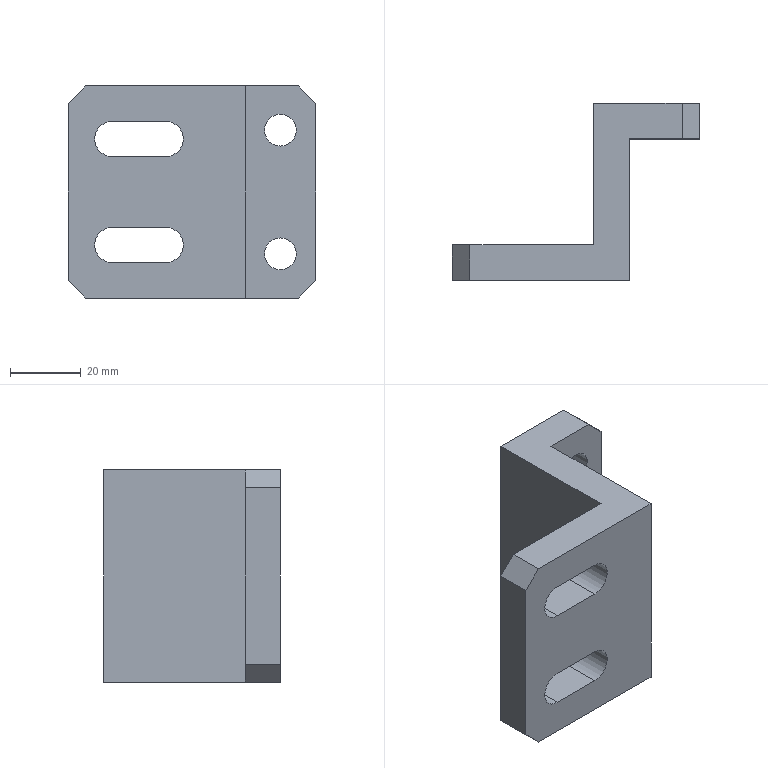Part | SolidWorks | features HoleWzd 2, Chamfer 1, Extrusion 1 | 1 solid | 26 faces | box 70 x 50 x 60 mm | volume 59657 mm3 | plane 18 | cylinder 8 | commonest cylinder face diameters 9 x4 10 x4
STEP:
#1=CARTESIAN_POINT('',(10.,40.,-22.));
#2=VERTEX_POINT('',#1);
#3=CARTESIAN_POINT('',(10.,40.,-13.));
#4=VERTEX_POINT('',#3);
#5=CARTESIAN_POINT('',(10.,40.,-17.5));
#6=DIRECTION('',(0.,1.,0.));
#7=DIRECTION('',(0.,0.,1.));
#8=AXIS2_PLACEMENT_3D('',#5,#6,#7);
#9=CIRCLE('',#8,4.5);
#10=EDGE_CURVE('',#2,#4,#9,.T.);
#11=ORIENTED_EDGE('',*,*,#10,.F.);
#12=CARTESIAN_POINT('',(10.,50.,-22.));
#13=VERTEX_POINT('',#12);
#14=CARTESIAN_POINT('',(10.,50.,-22.));
#15=DIRECTION('',(0.,1.,0.));
#16=VECTOR('',#15,1000.);
#17=LINE('',#14,#16);
#18=EDGE_CURVE('',#2,#13,#17,.T.);
#19=ORIENTED_EDGE('',*,*,#18,.T.);
#20=CARTESIAN_POINT('',(10.,50.,-13.));
#21=VERTEX_POINT('',#20);
#22=CARTESIAN_POINT('',(10.,50.,-17.5));
#23=DIRECTION('',(0.,1.,0.));
#24=DIRECTION('',(0.,0.,1.));
#25=AXIS2_PLACEMENT_3D('',#22,#23,#24);
#26=CIRCLE('',#25,4.5);
#27=EDGE_CURVE('',#13,#21,#26,.T.);
#28=ORIENTED_EDGE('',*,*,#27,.T.);
#29=CARTESIAN_POINT('',(10.,50.,-13.));
#30=DIRECTION('',(0.,1.,0.));
#31=VECTOR('',#30,1000.);
#32=LINE('',#29,#31);
#33=EDGE_CURVE('',#4,#21,#32,.T.);
#34=ORIENTED_EDGE('',*,*,#33,.F.);
#35=EDGE_LOOP('',(#11,#19,#28,#34));
#36=FACE_OUTER_BOUND('',#35,.T.);
#37=CARTESIAN_POINT('',(10.,50.,-17.5));
#38=DIRECTION('',(0.,1.,0.));
#39=DIRECTION('',(0.,0.,1.));
#40=AXIS2_PLACEMENT_3D('',#37,#38,#39);
#41=CYLINDRICAL_SURFACE('',#40,4.5);
#42=ADVANCED_FACE('',(#36),#41,.F.);
#43=CARTESIAN_POINT('',(10.,40.,13.));
#44=VERTEX_POINT('',#43);
#45=CARTESIAN_POINT('',(10.,40.,22.));
#46=VERTEX_POINT('',#45);
#47=CARTESIAN_POINT('',(10.,40.,17.5));
#48=DIRECTION('',(0.,1.,0.));
#49=DIRECTION('',(0.,0.,1.));
#50=AXIS2_PLACEMENT_3D('',#47,#48,#49);
#51=CIRCLE('',#50,4.5);
#52=EDGE_CURVE('',#44,#46,#51,.T.);
#53=ORIENTED_EDGE('',*,*,#52,.F.);
#54=CARTESIAN_POINT('',(10.,50.,13.));
#55=VERTEX_POINT('',#54);
#56=CARTESIAN_POINT('',(10.,50.,13.));
#57=DIRECTION('',(0.,1.,0.));
#58=VECTOR('',#57,1000.);
#59=LINE('',#56,#58);
#60=EDGE_CURVE('',#44,#55,#59,.T.);
#61=ORIENTED_EDGE('',*,*,#60,.T.);
#62=CARTESIAN_POINT('',(10.,50.,22.));
#63=VERTEX_POINT('',#62);
#64=CARTESIAN_POINT('',(10.,50.,17.5));
#65=DIRECTION('',(0.,1.,0.));
#66=DIRECTION('',(0.,0.,1.));
#67=AXIS2_PLACEMENT_3D('',#64,#65,#66);
#68=CIRCLE('',#67,4.5);
#69=EDGE_CURVE('',#55,#63,#68,.T.);
#70=ORIENTED_EDGE('',*,*,#69,.T.);
#71=CARTESIAN_POINT('',(10.,50.,22.));
#72=DIRECTION('',(0.,1.,0.));
#73=VECTOR('',#72,1000.);
#74=LINE('',#71,#73);
#75=EDGE_CURVE('',#46,#63,#74,.T.);
#76=ORIENTED_EDGE('',*,*,#75,.F.);
#77=EDGE_LOOP('',(#53,#61,#70,#76));
#78=FACE_OUTER_BOUND('',#77,.T.);
#79=CARTESIAN_POINT('',(10.,50.,17.5));
#80=DIRECTION('',(0.,1.,0.));
#81=DIRECTION('',(0.,0.,1.));
#82=AXIS2_PLACEMENT_3D('',#79,#80,#81);
#83=CYLINDRICAL_SURFACE('',#82,4.5);
#84=ADVANCED_FACE('',(#78),#83,.F.);
#85=CARTESIAN_POINT('',(-45.,0.,30.));
#86=VERTEX_POINT('',#85);
#87=CARTESIAN_POINT('',(0.,0.,30.));
#88=VERTEX_POINT('',#87);
#89=CARTESIAN_POINT('',(0.,0.,30.));
#90=DIRECTION('',(1.,0.,0.));
#91=VECTOR('',#90,1000.);
#92=LINE('',#89,#91);
#93=EDGE_CURVE('',#86,#88,#92,.T.);
#94=ORIENTED_EDGE('',*,*,#93,.F.);
#95=CARTESIAN_POINT('',(-50.,0.,25.));
#96=VERTEX_POINT('',#95);
#97=CARTESIAN_POINT('',(-45.,0.,30.));
#98=DIRECTION('',(-0.7071,0.,-0.7071));
#99=VECTOR('',#98,1000.);
#100=LINE('',#97,#99);
#101=EDGE_CURVE('',#86,#96,#100,.T.);
#102=ORIENTED_EDGE('',*,*,#101,.T.);
#103=CARTESIAN_POINT('',(-50.,0.,-25.));
#104=VERTEX_POINT('',#103);
#105=CARTESIAN_POINT('',(-50.,0.,30.));
#106=DIRECTION('',(0.,0.,-1.));
#107=VECTOR('',#106,1000.);
#108=LINE('',#105,#107);
#109=EDGE_CURVE('',#96,#104,#108,.T.);
#110=ORIENTED_EDGE('',*,*,#109,.T.);
#111=CARTESIAN_POINT('',(-45.,0.,-30.));
#112=VERTEX_POINT('',#111);
#113=CARTESIAN_POINT('',(-50.,0.,-25.));
#114=DIRECTION('',(0.7071,0.,-0.7071));
#115=VECTOR('',#114,1000.);
#116=LINE('',#113,#115);
#117=EDGE_CURVE('',#104,#112,#116,.T.);
#118=ORIENTED_EDGE('',*,*,#117,.T.);
#119=CARTESIAN_POINT('',(0.,0.,-30.));
#120=VERTEX_POINT('',#119);
#121=CARTESIAN_POINT('',(0.,0.,-30.));
#122=DIRECTION('',(1.,0.,0.));
#123=VECTOR('',#122,1000.);
#124=LINE('',#121,#123);
#125=EDGE_CURVE('',#112,#120,#124,.T.);
#126=ORIENTED_EDGE('',*,*,#125,.T.);
#127=CARTESIAN_POINT('',(0.,0.,30.));
#128=DIRECTION('',(0.,0.,-1.));
#129=VECTOR('',#128,1000.);
#130=LINE('',#127,#129);
#131=EDGE_CURVE('',#88,#120,#130,.T.);
#132=ORIENTED_EDGE('',*,*,#131,.F.);
#133=EDGE_LOOP('',(#94,#102,#110,#118,#126,#132));
#134=FACE_OUTER_BOUND('',#133,.T.);
#135=CARTESIAN_POINT('',(-37.5,0.,10.));
#136=VERTEX_POINT('',#135);
#137=CARTESIAN_POINT('',(-22.5,0.,10.));
#138=VERTEX_POINT('',#137);
#139=CARTESIAN_POINT('',(-37.5,0.,10.));
#140=DIRECTION('',(1.,0.,0.));
#141=VECTOR('',#140,1000.);
#142=LINE('',#139,#141);
#143=EDGE_CURVE('',#136,#138,#142,.T.);
#144=ORIENTED_EDGE('',*,*,#143,.F.);
#145=CARTESIAN_POINT('',(-37.5,0.,20.));
#146=VERTEX_POINT('',#145);
#147=CARTESIAN_POINT('',(-37.5,0.,15.));
#148=DIRECTION('',(0.,1.,0.));
#149=DIRECTION('',(0.,0.,1.));
#150=AXIS2_PLACEMENT_3D('',#147,#148,#149);
#151=CIRCLE('',#150,5.);
#152=EDGE_CURVE('',#136,#146,#151,.T.);
#153=ORIENTED_EDGE('',*,*,#152,.T.);
#154=CARTESIAN_POINT('',(-22.5,0.,20.));
#155=VERTEX_POINT('',#154);
#156=CARTESIAN_POINT('',(-37.5,0.,20.));
#157=DIRECTION('',(1.,0.,0.));
#158=VECTOR('',#157,1000.);
#159=LINE('',#156,#158);
#160=EDGE_CURVE('',#146,#155,#159,.T.);
#161=ORIENTED_EDGE('',*,*,#160,.T.);
#162=CARTESIAN_POINT('',(-22.5,0.,15.));
#163=DIRECTION('',(0.,1.,0.));
#164=DIRECTION('',(0.,0.,1.));
#165=AXIS2_PLACEMENT_3D('',#162,#163,#164);
#166=CIRCLE('',#165,5.);
#167=EDGE_CURVE('',#155,#138,#166,.T.);
#168=ORIENTED_EDGE('',*,*,#167,.T.);
#169=EDGE_LOOP('',(#144,#153,#161,#168));
#170=FACE_BOUND('',#169,.T.);
#171=CARTESIAN_POINT('',(-37.5,0.,-20.));
#172=VERTEX_POINT('',#171);
#173=CARTESIAN_POINT('',(-22.5,0.,-20.));
#174=VERTEX_POINT('',#173);
#175=CARTESIAN_POINT('',(-37.5,0.,-20.));
#176=DIRECTION('',(1.,0.,0.));
#177=VECTOR('',#176,1000.);
#178=LINE('',#175,#177);
#179=EDGE_CURVE('',#172,#174,#178,.T.);
#180=ORIENTED_EDGE('',*,*,#179,.F.);
#181=CARTESIAN_POINT('',(-37.5,0.,-10.));
#182=VERTEX_POINT('',#181);
#183=CARTESIAN_POINT('',(-37.5,0.,-15.));
#184=DIRECTION('',(0.,1.,0.));
#185=DIRECTION('',(0.,0.,1.));
#186=AXIS2_PLACEMENT_3D('',#183,#184,#185);
#187=CIRCLE('',#186,5.);
#188=EDGE_CURVE('',#172,#182,#187,.T.);
#189=ORIENTED_EDGE('',*,*,#188,.T.);
#190=CARTESIAN_POINT('',(-22.5,0.,-10.));
#191=VERTEX_POINT('',#190);
#192=CARTESIAN_POINT('',(-37.5,0.,-10.));
#193=DIRECTION('',(1.,0.,0.));
#194=VECTOR('',#193,1000.);
#195=LINE('',#192,#194);
#196=EDGE_CURVE('',#182,#191,#195,.T.);
#197=ORIENTED_EDGE('',*,*,#196,.T.);
#198=CARTESIAN_POINT('',(-22.5,0.,-15.));
#199=DIRECTION('',(0.,1.,0.));
#200=DIRECTION('',(0.,0.,1.));
#201=AXIS2_PLACEMENT_3D('',#198,#199,#200);
#202=CIRCLE('',#201,5.);
#203=EDGE_CURVE('',#191,#174,#202,.T.);
#204=ORIENTED_EDGE('',*,*,#203,.T.);
#205=EDGE_LOOP('',(#180,#189,#197,#204));
#206=FACE_BOUND('',#205,.T.);
#207=CARTESIAN_POINT('',(0.,0.,30.));
#208=DIRECTION('',(0.,1.,0.));
#209=DIRECTION('',(-1.,0.,0.));
#210=AXIS2_PLACEMENT_3D('',#207,#208,#209);
#211=PLANE('',#210);
#212=ADVANCED_FACE('',(#134,#170,#206),#211,.F.);
#213=CARTESIAN_POINT('',(-50.,10.,25.));
#214=VERTEX_POINT('',#213);
#215=CARTESIAN_POINT('',(-50.,10.,-25.));
#216=VERTEX_POINT('',#215);
#217=CARTESIAN_POINT('',(-50.,10.,30.));
#218=DIRECTION('',(0.,0.,-1.));
#219=VECTOR('',#218,1000.);
#220=LINE('',#217,#219);
#221=EDGE_CURVE('',#214,#216,#220,.T.);
#222=ORIENTED_EDGE('',*,*,#221,.F.);
#223=CARTESIAN_POINT('',(-45.,10.,30.));
#224=VERTEX_POINT('',#223);
#225=CARTESIAN_POINT('',(-45.,10.,30.));
#226=DIRECTION('',(0.7071,0.,0.7071));
#227=VECTOR('',#226,1000.);
#228=LINE('',#225,#227);
#229=EDGE_CURVE('',#214,#224,#228,.T.);
#230=ORIENTED_EDGE('',*,*,#229,.T.);
#231=CARTESIAN_POINT('',(-10.,10.,30.));
#232=VERTEX_POINT('',#231);
#233=CARTESIAN_POINT('',(-10.,10.,30.));
#234=DIRECTION('',(-1.,0.,0.));
#235=VECTOR('',#234,1000.);
#236=LINE('',#233,#235);
#237=EDGE_CURVE('',#232,#224,#236,.T.);
#238=ORIENTED_EDGE('',*,*,#237,.F.);
#239=CARTESIAN_POINT('',(-10.,10.,-30.));
#240=VERTEX_POINT('',#239);
#241=CARTESIAN_POINT('',(-10.,10.,30.));
#242=DIRECTION('',(0.,0.,-1.));
#243=VECTOR('',#242,1000.);
#244=LINE('',#241,#243);
#245=EDGE_CURVE('',#232,#240,#244,.T.);
#246=ORIENTED_EDGE('',*,*,#245,.T.);
#247=CARTESIAN_POINT('',(-45.,10.,-30.));
#248=VERTEX_POINT('',#247);
#249=CARTESIAN_POINT('',(-10.,10.,-30.));
#250=DIRECTION('',(-1.,0.,0.));
#251=VECTOR('',#250,1000.);
#252=LINE('',#249,#251);
#253=EDGE_CURVE('',#240,#248,#252,.T.);
#254=ORIENTED_EDGE('',*,*,#253,.T.);
#255=CARTESIAN_POINT('',(-50.,10.,-25.));
#256=DIRECTION('',(-0.7071,0.,0.7071));
#257=VECTOR('',#256,1000.);
#258=LINE('',#255,#257);
#259=EDGE_CURVE('',#248,#216,#258,.T.);
#260=ORIENTED_EDGE('',*,*,#259,.T.);
#261=EDGE_LOOP('',(#222,#230,#238,#246,#254,#260));
#262=FACE_OUTER_BOUND('',#261,.T.);
#263=CARTESIAN_POINT('',(-37.5,10.,10.));
#264=VERTEX_POINT('',#263);
#265=CARTESIAN_POINT('',(-22.5,10.,10.));
#266=VERTEX_POINT('',#265);
#267=CARTESIAN_POINT('',(-37.5,10.,10.));
#268=DIRECTION('',(1.,0.,0.));
#269=VECTOR('',#268,1000.);
#270=LINE('',#267,#269);
#271=EDGE_CURVE('',#264,#266,#270,.T.);
#272=ORIENTED_EDGE('',*,*,#271,.T.);
#273=CARTESIAN_POINT('',(-22.5,10.,20.));
#274=VERTEX_POINT('',#273);
#275=CARTESIAN_POINT('',(-22.5,10.,15.));
#276=DIRECTION('',(0.,1.,0.));
#277=DIRECTION('',(0.,0.,1.));
#278=AXIS2_PLACEMENT_3D('',#275,#276,#277);
#279=CIRCLE('',#278,5.);
#280=EDGE_CURVE('',#274,#266,#279,.T.);
#281=ORIENTED_EDGE('',*,*,#280,.F.);
#282=CARTESIAN_POINT('',(-37.5,10.,20.));
#283=VERTEX_POINT('',#282);
#284=CARTESIAN_POINT('',(-37.5,10.,20.));
#285=DIRECTION('',(1.,0.,0.));
#286=VECTOR('',#285,1000.);
#287=LINE('',#284,#286);
#288=EDGE_CURVE('',#283,#274,#287,.T.);
#289=ORIENTED_EDGE('',*,*,#288,.F.);
#290=CARTESIAN_POINT('',(-37.5,10.,15.));
#291=DIRECTION('',(0.,1.,0.));
#292=DIRECTION('',(0.,0.,1.));
#293=AXIS2_PLACEMENT_3D('',#290,#291,#292);
#294=CIRCLE('',#293,5.);
#295=EDGE_CURVE('',#264,#283,#294,.T.);
#296=ORIENTED_EDGE('',*,*,#295,.F.);
#297=EDGE_LOOP('',(#272,#281,#289,#296));
#298=FACE_BOUND('',#297,.T.);
#299=CARTESIAN_POINT('',(-37.5,10.,-20.));
#300=VERTEX_POINT('',#299);
#301=CARTESIAN_POINT('',(-37.5,10.,-10.));
#302=VERTEX_POINT('',#301);
#303=CARTESIAN_POINT('',(-37.5,10.,-15.));
#304=DIRECTION('',(0.,1.,0.));
#305=DIRECTION('',(0.,0.,1.));
#306=AXIS2_PLACEMENT_3D('',#303,#304,#305);
#307=CIRCLE('',#306,5.);
#308=EDGE_CURVE('',#300,#302,#307,.T.);
#309=ORIENTED_EDGE('',*,*,#308,.F.);
#310=CARTESIAN_POINT('',(-22.5,10.,-20.));
#311=VERTEX_POINT('',#310);
#312=CARTESIAN_POINT('',(-37.5,10.,-20.));
#313=DIRECTION('',(1.,0.,0.));
#314=VECTOR('',#313,1000.);
#315=LINE('',#312,#314);
#316=EDGE_CURVE('',#300,#311,#315,.T.);
#317=ORIENTED_EDGE('',*,*,#316,.T.);
#318=CARTESIAN_POINT('',(-22.5,10.,-10.));
#319=VERTEX_POINT('',#318);
#320=CARTESIAN_POINT('',(-22.5,10.,-15.));
#321=DIRECTION('',(0.,1.,0.));
#322=DIRECTION('',(0.,0.,1.));
#323=AXIS2_PLACEMENT_3D('',#320,#321,#322);
#324=CIRCLE('',#323,5.);
#325=EDGE_CURVE('',#319,#311,#324,.T.);
#326=ORIENTED_EDGE('',*,*,#325,.F.);
#327=CARTESIAN_POINT('',(-37.5,10.,-10.));
#328=DIRECTION('',(1.,0.,0.));
#329=VECTOR('',#328,1000.);
#330=LINE('',#327,#329);
#331=EDGE_CURVE('',#302,#319,#330,.T.);
#332=ORIENTED_EDGE('',*,*,#331,.F.);
#333=EDGE_LOOP('',(#309,#317,#326,#332));
#334=FACE_BOUND('',#333,.T.);
#335=CARTESIAN_POINT('',(-10.,10.,30.));
#336=DIRECTION('',(0.,-1.,0.));
#337=DIRECTION('',(1.,0.,0.));
#338=AXIS2_PLACEMENT_3D('',#335,#336,#337);
#339=PLANE('',#338);
#340=ADVANCED_FACE('',(#262,#298,#334),#339,.F.);
#341=CARTESIAN_POINT('',(0.,40.,-30.));
#342=VERTEX_POINT('',#341);
#343=CARTESIAN_POINT('',(0.,0.,-30.));
#344=DIRECTION('',(0.,1.,0.));
#345=VECTOR('',#344,1000.);
#346=LINE('',#343,#345);
#347=EDGE_CURVE('',#120,#342,#346,.T.);
#348=ORIENTED_EDGE('',*,*,#347,.T.);
#349=CARTESIAN_POINT('',(0.,40.,30.));
#350=VERTEX_POINT('',#349);
#351=CARTESIAN_POINT('',(0.,40.,30.));
#352=DIRECTION('',(0.,0.,-1.));
#353=VECTOR('',#352,1000.);
#354=LINE('',#351,#353);
#355=EDGE_CURVE('',#350,#342,#354,.T.);
#356=ORIENTED_EDGE('',*,*,#355,.F.);
#357=CARTESIAN_POINT('',(0.,0.,30.));
#358=DIRECTION('',(0.,1.,0.));
#359=VECTOR('',#358,1000.);
#360=LINE('',#357,#359);
#361=EDGE_CURVE('',#88,#350,#360,.T.);
#362=ORIENTED_EDGE('',*,*,#361,.F.);
#363=ORIENTED_EDGE('',*,*,#131,.T.);
#364=EDGE_LOOP('',(#348,#356,#362,#363));
#365=FACE_OUTER_BOUND('',#364,.T.);
#366=CARTESIAN_POINT('',(0.,0.,30.));
#367=DIRECTION('',(-1.,0.,0.));
#368=DIRECTION('',(0.,0.,1.));
#369=AXIS2_PLACEMENT_3D('',#366,#367,#368);
#370=PLANE('',#369);
#371=ADVANCED_FACE('',(#365),#370,.F.);
#372=CARTESIAN_POINT('',(10.,40.,-17.5));
#373=DIRECTION('',(0.,1.,0.));
#374=DIRECTION('',(0.,0.,1.));
#375=AXIS2_PLACEMENT_3D('',#372,#373,#374);
#376=CIRCLE('',#375,4.5);
#377=EDGE_CURVE('',#4,#2,#376,.T.);
#378=ORIENTED_EDGE('',*,*,#377,.T.);
#379=ORIENTED_EDGE('',*,*,#10,.T.);
#380=EDGE_LOOP('',(#378,#379));
#381=FACE_BOUND('',#380,.T.);
#382=CARTESIAN_POINT('',(10.,40.,17.5));
#383=DIRECTION('',(0.,1.,0.));
#384=DIRECTION('',(0.,0.,1.));
#385=AXIS2_PLACEMENT_3D('',#382,#383,#384);
#386=CIRCLE('',#385,4.5);
#387=EDGE_CURVE('',#46,#44,#386,.T.);
#388=ORIENTED_EDGE('',*,*,#387,.T.);
#389=ORIENTED_EDGE('',*,*,#52,.T.);
#390=EDGE_LOOP('',(#388,#389));
#391=FACE_BOUND('',#390,.T.);
#392=CARTESIAN_POINT('',(15.,40.,-30.));
#393=VERTEX_POINT('',#392);
#394=CARTESIAN_POINT('',(0.,40.,-30.));
#395=DIRECTION('',(1.,0.,0.));
#396=VECTOR('',#395,1000.);
#397=LINE('',#394,#396);
#398=EDGE_CURVE('',#342,#393,#397,.T.);
#399=ORIENTED_EDGE('',*,*,#398,.T.);
#400=CARTESIAN_POINT('',(20.,40.,-25.));
#401=VERTEX_POINT('',#400);
#402=CARTESIAN_POINT('',(20.,40.,-25.));
#403=DIRECTION('',(0.7071,0.,0.7071));
#404=VECTOR('',#403,1000.);
#405=LINE('',#402,#404);
#406=EDGE_CURVE('',#393,#401,#405,.T.);
#407=ORIENTED_EDGE('',*,*,#406,.T.);
#408=CARTESIAN_POINT('',(20.,40.,25.));
#409=VERTEX_POINT('',#408);
#410=CARTESIAN_POINT('',(20.,40.,30.));
#411=DIRECTION('',(0.,0.,-1.));
#412=VECTOR('',#411,1000.);
#413=LINE('',#410,#412);
#414=EDGE_CURVE('',#409,#401,#413,.T.);
#415=ORIENTED_EDGE('',*,*,#414,.F.);
#416=CARTESIAN_POINT('',(15.,40.,30.));
#417=VERTEX_POINT('',#416);
#418=CARTESIAN_POINT('',(15.,40.,30.));
#419=DIRECTION('',(-0.7071,0.,0.7071));
#420=VECTOR('',#419,1000.);
#421=LINE('',#418,#420);
#422=EDGE_CURVE('',#409,#417,#421,.T.);
#423=ORIENTED_EDGE('',*,*,#422,.T.);
#424=CARTESIAN_POINT('',(0.,40.,30.));
#425=DIRECTION('',(1.,0.,0.));
#426=VECTOR('',#425,1000.);
#427=LINE('',#424,#426);
#428=EDGE_CURVE('',#350,#417,#427,.T.);
#429=ORIENTED_EDGE('',*,*,#428,.F.);
#430=ORIENTED_EDGE('',*,*,#355,.T.);
#431=EDGE_LOOP('',(#399,#407,#415,#423,#429,#430));
#432=FACE_OUTER_BOUND('',#431,.T.);
#433=CARTESIAN_POINT('',(0.,40.,30.));
#434=DIRECTION('',(0.,1.,0.));
#435=DIRECTION('',(0.,0.,1.));
#436=AXIS2_PLACEMENT_3D('',#433,#434,#435);
#437=PLANE('',#436);
#438=ADVANCED_FACE('',(#381,#391,#432),#437,.F.);
#439=ORIENTED_EDGE('',*,*,#414,.T.);
#440=CARTESIAN_POINT('',(20.,50.,-25.));
#441=VERTEX_POINT('',#440);
#442=CARTESIAN_POINT('',(20.,50.,-25.));
#443=DIRECTION('',(0.,1.,0.));
#444=VECTOR('',#443,1000.);
#445=LINE('',#442,#444);
#446=EDGE_CURVE('',#401,#441,#445,.T.);
#447=ORIENTED_EDGE('',*,*,#446,.T.);
#448=CARTESIAN_POINT('',(20.,50.,25.));
#449=VERTEX_POINT('',#448);
#450=CARTESIAN_POINT('',(20.,50.,30.));
#451=DIRECTION('',(0.,0.,-1.));
#452=VECTOR('',#451,1000.);
#453=LINE('',#450,#452);
#454=EDGE_CURVE('',#449,#441,#453,.T.);
#455=ORIENTED_EDGE('',*,*,#454,.F.);
#456=CARTESIAN_POINT('',(20.,40.,25.));
#457=DIRECTION('',(0.,-1.,0.));
#458=VECTOR('',#457,1000.);
#459=LINE('',#456,#458);
#460=EDGE_CURVE('',#449,#409,#459,.T.);
#461=ORIENTED_EDGE('',*,*,#460,.T.);
#462=EDGE_LOOP('',(#439,#447,#455,#461));
#463=FACE_OUTER_BOUND('',#462,.T.);
#464=CARTESIAN_POINT('',(20.,50.,30.));
#465=DIRECTION('',(-1.,0.,0.));
#466=DIRECTION('',(0.,0.,1.));
#467=AXIS2_PLACEMENT_3D('',#464,#465,#466);
#468=PLANE('',#467);
#469=ADVANCED_FACE('',(#463),#468,.F.);
#470=CARTESIAN_POINT('',(10.,50.,-17.5));
#471=DIRECTION('',(0.,1.,0.));
#472=DIRECTION('',(0.,0.,1.));
#473=AXIS2_PLACEMENT_3D('',#470,#471,#472);
#474=CIRCLE('',#473,4.5);
#475=EDGE_CURVE('',#21,#13,#474,.T.);
#476=ORIENTED_EDGE('',*,*,#475,.F.);
#477=ORIENTED_EDGE('',*,*,#27,.F.);
#478=EDGE_LOOP('',(#476,#477));
#479=FACE_BOUND('',#478,.T.);
#480=CARTESIAN_POINT('',(10.,50.,17.5));
#481=DIRECTION('',(0.,1.,0.));
#482=DIRECTION('',(0.,0.,1.));
#483=AXIS2_PLACEMENT_3D('',#480,#481,#482);
#484=CIRCLE('',#483,4.5);
#485=EDGE_CURVE('',#63,#55,#484,.T.);
#486=ORIENTED_EDGE('',*,*,#485,.F.);
#487=ORIENTED_EDGE('',*,*,#69,.F.);
#488=EDGE_LOOP('',(#486,#487));
#489=FACE_BOUND('',#488,.T.);
#490=ORIENTED_EDGE('',*,*,#454,.T.);
#491=CARTESIAN_POINT('',(15.,50.,-30.));
#492=VERTEX_POINT('',#491);
#493=CARTESIAN_POINT('',(20.,50.,-25.));
#494=DIRECTION('',(-0.7071,0.,-0.7071));
#495=VECTOR('',#494,1000.);
#496=LINE('',#493,#495);
#497=EDGE_CURVE('',#441,#492,#496,.T.);
#498=ORIENTED_EDGE('',*,*,#497,.T.);
#499=CARTESIAN_POINT('',(-10.,50.,-30.));
#500=VERTEX_POINT('',#499);
#501=CARTESIAN_POINT('',(-10.,50.,-30.));
#502=DIRECTION('',(-1.,0.,0.));
#503=VECTOR('',#502,1000.);
#504=LINE('',#501,#503);
#505=EDGE_CURVE('',#492,#500,#504,.T.);
#506=ORIENTED_EDGE('',*,*,#505,.T.);
#507=CARTESIAN_POINT('',(-10.,50.,30.));
#508=VERTEX_POINT('',#507);
#509=CARTESIAN_POINT('',(-10.,50.,30.));
#510=DIRECTION('',(0.,0.,-1.));
#511=VECTOR('',#510,1000.);
#512=LINE('',#509,#511);
#513=EDGE_CURVE('',#508,#500,#512,.T.);
#514=ORIENTED_EDGE('',*,*,#513,.F.);
#515=CARTESIAN_POINT('',(15.,50.,30.));
#516=VERTEX_POINT('',#515);
#517=CARTESIAN_POINT('',(-10.,50.,30.));
#518=DIRECTION('',(-1.,0.,0.));
#519=VECTOR('',#518,1000.);
#520=LINE('',#517,#519);
#521=EDGE_CURVE('',#516,#508,#520,.T.);
#522=ORIENTED_EDGE('',*,*,#521,.F.);
#523=CARTESIAN_POINT('',(15.,50.,30.));
#524=DIRECTION('',(0.7071,0.,-0.7071));
#525=VECTOR('',#524,1000.);
#526=LINE('',#523,#525);
#527=EDGE_CURVE('',#516,#449,#526,.T.);
#528=ORIENTED_EDGE('',*,*,#527,.T.);
#529=EDGE_LOOP('',(#490,#498,#506,#514,#522,#528));
#530=FACE_OUTER_BOUND('',#529,.T.);
#531=CARTESIAN_POINT('',(-10.,50.,30.));
#532=DIRECTION('',(0.,-1.,0.));
#533=DIRECTION('',(0.,0.,-1.));
#534=AXIS2_PLACEMENT_3D('',#531,#532,#533);
#535=PLANE('',#534);
#536=ADVANCED_FACE('',(#479,#489,#530),#535,.F.);
#537=CARTESIAN_POINT('',(-10.,10.,-30.));
#538=DIRECTION('',(0.,-1.,0.));
#539=VECTOR('',#538,1000.);
#540=LINE('',#537,#539);
#541=EDGE_CURVE('',#500,#240,#540,.T.);
#542=ORIENTED_EDGE('',*,*,#541,.T.);
#543=ORIENTED_EDGE('',*,*,#245,.F.);
#544=CARTESIAN_POINT('',(-10.,10.,30.));
#545=DIRECTION('',(0.,-1.,0.));
#546=VECTOR('',#545,1000.);
#547=LINE('',#544,#546);
#548=EDGE_CURVE('',#508,#232,#547,.T.);
#549=ORIENTED_EDGE('',*,*,#548,.F.);
#550=ORIENTED_EDGE('',*,*,#513,.T.);
#551=EDGE_LOOP('',(#542,#543,#549,#550));
#552=FACE_OUTER_BOUND('',#551,.T.);
#553=CARTESIAN_POINT('',(-10.,10.,30.));
#554=DIRECTION('',(1.,0.,0.));
#555=DIRECTION('',(0.,0.,-1.));
#556=AXIS2_PLACEMENT_3D('',#553,#554,#555);
#557=PLANE('',#556);
#558=ADVANCED_FACE('',(#552),#557,.F.);
#559=ORIENTED_EDGE('',*,*,#109,.F.);
#560=CARTESIAN_POINT('',(-50.,10.,25.));
#561=DIRECTION('',(0.,1.,0.));
#562=VECTOR('',#561,1000.);
#563=LINE('',#560,#562);
#564=EDGE_CURVE('',#96,#214,#563,.T.);
#565=ORIENTED_EDGE('',*,*,#564,.T.);
#566=ORIENTED_EDGE('',*,*,#221,.T.);
#567=CARTESIAN_POINT('',(-50.,10.,-25.));
#568=DIRECTION('',(0.,-1.,0.));
#569=VECTOR('',#568,1000.);
#570=LINE('',#567,#569);
#571=EDGE_CURVE('',#216,#104,#570,.T.);
#572=ORIENTED_EDGE('',*,*,#571,.T.);
#573=EDGE_LOOP('',(#559,#565,#566,#572));
#574=FACE_OUTER_BOUND('',#573,.T.);
#575=CARTESIAN_POINT('',(-50.,10.,30.));
#576=DIRECTION('',(1.,0.,0.));
#577=DIRECTION('',(0.,0.,-1.));
#578=AXIS2_PLACEMENT_3D('',#575,#576,#577);
#579=PLANE('',#578);
#580=ADVANCED_FACE('',(#574),#579,.F.);
#581=ORIENTED_EDGE('',*,*,#237,.T.);
#582=CARTESIAN_POINT('',(-45.,0.,30.));
#583=DIRECTION('',(0.,-1.,0.));
#584=VECTOR('',#583,1000.);
#585=LINE('',#582,#584);
#586=EDGE_CURVE('',#224,#86,#585,.T.);
#587=ORIENTED_EDGE('',*,*,#586,.T.);
#588=ORIENTED_EDGE('',*,*,#93,.T.);
#589=ORIENTED_EDGE('',*,*,#361,.T.);
#590=ORIENTED_EDGE('',*,*,#428,.T.);
#591=CARTESIAN_POINT('',(15.,50.,30.));
#592=DIRECTION('',(0.,1.,0.));
#593=VECTOR('',#592,1000.);
#594=LINE('',#591,#593);
#595=EDGE_CURVE('',#417,#516,#594,.T.);
#596=ORIENTED_EDGE('',*,*,#595,.T.);
#597=ORIENTED_EDGE('',*,*,#521,.T.);
#598=ORIENTED_EDGE('',*,*,#548,.T.);
#599=EDGE_LOOP('',(#581,#587,#588,#589,#590,#596,#597,#598));
#600=FACE_OUTER_BOUND('',#599,.T.);
#601=CARTESIAN_POINT('',(0.,0.,30.));
#602=DIRECTION('',(0.,0.,1.));
#603=DIRECTION('',(1.,0.,0.));
#604=AXIS2_PLACEMENT_3D('',#601,#602,#603);
#605=PLANE('',#604);
#606=ADVANCED_FACE('',(#600),#605,.T.);
#607=ORIENTED_EDGE('',*,*,#125,.F.);
#608=CARTESIAN_POINT('',(-45.,0.,-30.));
#609=DIRECTION('',(0.,1.,0.));
#610=VECTOR('',#609,1000.);
#611=LINE('',#608,#610);
#612=EDGE_CURVE('',#112,#248,#611,.T.);
#613=ORIENTED_EDGE('',*,*,#612,.T.);
#614=ORIENTED_EDGE('',*,*,#253,.F.);
#615=ORIENTED_EDGE('',*,*,#541,.F.);
#616=ORIENTED_EDGE('',*,*,#505,.F.);
#617=CARTESIAN_POINT('',(15.,0.,-30.));
#618=DIRECTION('',(0.,-1.,0.));
#619=VECTOR('',#618,1000.);
#620=LINE('',#617,#619);
#621=EDGE_CURVE('',#492,#393,#620,.T.);
#622=ORIENTED_EDGE('',*,*,#621,.T.);
#623=ORIENTED_EDGE('',*,*,#398,.F.);
#624=ORIENTED_EDGE('',*,*,#347,.F.);
#625=EDGE_LOOP('',(#607,#613,#614,#615,#616,#622,#623,#624));
#626=FACE_OUTER_BOUND('',#625,.T.);
#627=CARTESIAN_POINT('',(0.,0.,-30.));
#628=DIRECTION('',(0.,0.,1.));
#629=DIRECTION('',(1.,0.,0.));
#630=AXIS2_PLACEMENT_3D('',#627,#628,#629);
#631=PLANE('',#630);
#632=ADVANCED_FACE('',(#626),#631,.F.);
#633=ORIENTED_EDGE('',*,*,#60,.F.);
#634=ORIENTED_EDGE('',*,*,#387,.F.);
#635=ORIENTED_EDGE('',*,*,#75,.T.);
#636=ORIENTED_EDGE('',*,*,#485,.T.);
#637=EDGE_LOOP('',(#633,#634,#635,#636));
#638=FACE_OUTER_BOUND('',#637,.T.);
#639=CARTESIAN_POINT('',(10.,50.,17.5));
#640=DIRECTION('',(0.,1.,0.));
#641=DIRECTION('',(0.,0.,1.));
#642=AXIS2_PLACEMENT_3D('',#639,#640,#641);
#643=CYLINDRICAL_SURFACE('',#642,4.5);
#644=ADVANCED_FACE('',(#638),#643,.F.);
#645=ORIENTED_EDGE('',*,*,#18,.F.);
#646=ORIENTED_EDGE('',*,*,#377,.F.);
#647=ORIENTED_EDGE('',*,*,#33,.T.);
#648=ORIENTED_EDGE('',*,*,#475,.T.);
#649=EDGE_LOOP('',(#645,#646,#647,#648));
#650=FACE_OUTER_BOUND('',#649,.T.);
#651=CARTESIAN_POINT('',(10.,50.,-17.5));
#652=DIRECTION('',(0.,1.,0.));
#653=DIRECTION('',(0.,0.,1.));
#654=AXIS2_PLACEMENT_3D('',#651,#652,#653);
#655=CYLINDRICAL_SURFACE('',#654,4.5);
#656=ADVANCED_FACE('',(#650),#655,.F.);
#657=ORIENTED_EDGE('',*,*,#167,.F.);
#658=CARTESIAN_POINT('',(-22.5,10.,20.));
#659=DIRECTION('',(0.,-1.,0.));
#660=VECTOR('',#659,1000.);
#661=LINE('',#658,#660);
#662=EDGE_CURVE('',#274,#155,#661,.T.);
#663=ORIENTED_EDGE('',*,*,#662,.F.);
#664=ORIENTED_EDGE('',*,*,#280,.T.);
#665=CARTESIAN_POINT('',(-22.5,10.,10.));
#666=DIRECTION('',(0.,1.,0.));
#667=VECTOR('',#666,1000.);
#668=LINE('',#665,#667);
#669=EDGE_CURVE('',#138,#266,#668,.T.);
#670=ORIENTED_EDGE('',*,*,#669,.F.);
#671=EDGE_LOOP('',(#657,#663,#664,#670));
#672=FACE_OUTER_BOUND('',#671,.T.);
#673=CARTESIAN_POINT('',(-22.5,10.,15.));
#674=DIRECTION('',(0.,1.,0.));
#675=DIRECTION('',(0.,0.,1.));
#676=AXIS2_PLACEMENT_3D('',#673,#674,#675);
#677=CYLINDRICAL_SURFACE('',#676,5.);
#678=ADVANCED_FACE('',(#672),#677,.F.);
#679=ORIENTED_EDGE('',*,*,#295,.T.);
#680=CARTESIAN_POINT('',(-37.5,10.,20.));
#681=DIRECTION('',(0.,1.,0.));
#682=VECTOR('',#681,1000.);
#683=LINE('',#680,#682);
#684=EDGE_CURVE('',#146,#283,#683,.T.);
#685=ORIENTED_EDGE('',*,*,#684,.F.);
#686=ORIENTED_EDGE('',*,*,#152,.F.);
#687=CARTESIAN_POINT('',(-37.5,10.,10.));
#688=DIRECTION('',(0.,-1.,0.));
#689=VECTOR('',#688,1000.);
#690=LINE('',#687,#689);
#691=EDGE_CURVE('',#264,#136,#690,.T.);
#692=ORIENTED_EDGE('',*,*,#691,.F.);
#693=EDGE_LOOP('',(#679,#685,#686,#692));
#694=FACE_OUTER_BOUND('',#693,.T.);
#695=CARTESIAN_POINT('',(-37.5,10.,15.));
#696=DIRECTION('',(0.,1.,0.));
#697=DIRECTION('',(0.,0.,1.));
#698=AXIS2_PLACEMENT_3D('',#695,#696,#697);
#699=CYLINDRICAL_SURFACE('',#698,5.);
#700=ADVANCED_FACE('',(#694),#699,.F.);
#701=ORIENTED_EDGE('',*,*,#669,.T.);
#702=ORIENTED_EDGE('',*,*,#271,.F.);
#703=ORIENTED_EDGE('',*,*,#691,.T.);
#704=ORIENTED_EDGE('',*,*,#143,.T.);
#705=EDGE_LOOP('',(#701,#702,#703,#704));
#706=FACE_OUTER_BOUND('',#705,.T.);
#707=CARTESIAN_POINT('',(-37.5,10.,10.));
#708=DIRECTION('',(0.,0.,-1.));
#709=DIRECTION('',(-1.,0.,0.));
#710=AXIS2_PLACEMENT_3D('',#707,#708,#709);
#711=PLANE('',#710);
#712=ADVANCED_FACE('',(#706),#711,.F.);
#713=ORIENTED_EDGE('',*,*,#662,.T.);
#714=ORIENTED_EDGE('',*,*,#160,.F.);
#715=ORIENTED_EDGE('',*,*,#684,.T.);
#716=ORIENTED_EDGE('',*,*,#288,.T.);
#717=EDGE_LOOP('',(#713,#714,#715,#716));
#718=FACE_OUTER_BOUND('',#717,.T.);
#719=CARTESIAN_POINT('',(-37.5,10.,20.));
#720=DIRECTION('',(0.,0.,1.));
#721=DIRECTION('',(1.,0.,0.));
#722=AXIS2_PLACEMENT_3D('',#719,#720,#721);
#723=PLANE('',#722);
#724=ADVANCED_FACE('',(#718),#723,.F.);
#725=ORIENTED_EDGE('',*,*,#203,.F.);
#726=CARTESIAN_POINT('',(-22.5,10.,-10.));
#727=DIRECTION('',(0.,-1.,0.));
#728=VECTOR('',#727,1000.);
#729=LINE('',#726,#728);
#730=EDGE_CURVE('',#319,#191,#729,.T.);
#731=ORIENTED_EDGE('',*,*,#730,.F.);
#732=ORIENTED_EDGE('',*,*,#325,.T.);
#733=CARTESIAN_POINT('',(-22.5,10.,-20.));
#734=DIRECTION('',(0.,1.,0.));
#735=VECTOR('',#734,1000.);
#736=LINE('',#733,#735);
#737=EDGE_CURVE('',#174,#311,#736,.T.);
#738=ORIENTED_EDGE('',*,*,#737,.F.);
#739=EDGE_LOOP('',(#725,#731,#732,#738));
#740=FACE_OUTER_BOUND('',#739,.T.);
#741=CARTESIAN_POINT('',(-22.5,10.,-15.));
#742=DIRECTION('',(0.,1.,0.));
#743=DIRECTION('',(0.,0.,1.));
#744=AXIS2_PLACEMENT_3D('',#741,#742,#743);
#745=CYLINDRICAL_SURFACE('',#744,5.);
#746=ADVANCED_FACE('',(#740),#745,.F.);
#747=ORIENTED_EDGE('',*,*,#308,.T.);
#748=CARTESIAN_POINT('',(-37.5,10.,-10.));
#749=DIRECTION('',(0.,1.,0.));
#750=VECTOR('',#749,1000.);
#751=LINE('',#748,#750);
#752=EDGE_CURVE('',#182,#302,#751,.T.);
#753=ORIENTED_EDGE('',*,*,#752,.F.);
#754=ORIENTED_EDGE('',*,*,#188,.F.);
#755=CARTESIAN_POINT('',(-37.5,10.,-20.));
#756=DIRECTION('',(0.,-1.,0.));
#757=VECTOR('',#756,1000.);
#758=LINE('',#755,#757);
#759=EDGE_CURVE('',#300,#172,#758,.T.);
#760=ORIENTED_EDGE('',*,*,#759,.F.);
#761=EDGE_LOOP('',(#747,#753,#754,#760));
#762=FACE_OUTER_BOUND('',#761,.T.);
#763=CARTESIAN_POINT('',(-37.5,10.,-15.));
#764=DIRECTION('',(0.,1.,0.));
#765=DIRECTION('',(0.,0.,1.));
#766=AXIS2_PLACEMENT_3D('',#763,#764,#765);
#767=CYLINDRICAL_SURFACE('',#766,5.);
#768=ADVANCED_FACE('',(#762),#767,.F.);
#769=ORIENTED_EDGE('',*,*,#737,.T.);
#770=ORIENTED_EDGE('',*,*,#316,.F.);
#771=ORIENTED_EDGE('',*,*,#759,.T.);
#772=ORIENTED_EDGE('',*,*,#179,.T.);
#773=EDGE_LOOP('',(#769,#770,#771,#772));
#774=FACE_OUTER_BOUND('',#773,.T.);
#775=CARTESIAN_POINT('',(-37.5,10.,-20.));
#776=DIRECTION('',(0.,0.,-1.));
#777=DIRECTION('',(-1.,0.,0.));
#778=AXIS2_PLACEMENT_3D('',#775,#776,#777);
#779=PLANE('',#778);
#780=ADVANCED_FACE('',(#774),#779,.F.);
#781=ORIENTED_EDGE('',*,*,#730,.T.);
#782=ORIENTED_EDGE('',*,*,#196,.F.);
#783=ORIENTED_EDGE('',*,*,#752,.T.);
#784=ORIENTED_EDGE('',*,*,#331,.T.);
#785=EDGE_LOOP('',(#781,#782,#783,#784));
#786=FACE_OUTER_BOUND('',#785,.T.);
#787=CARTESIAN_POINT('',(-37.5,10.,-10.));
#788=DIRECTION('',(0.,0.,1.));
#789=DIRECTION('',(1.,0.,0.));
#790=AXIS2_PLACEMENT_3D('',#787,#788,#789);
#791=PLANE('',#790);
#792=ADVANCED_FACE('',(#786),#791,.F.);
#793=ORIENTED_EDGE('',*,*,#229,.F.);
#794=ORIENTED_EDGE('',*,*,#564,.F.);
#795=ORIENTED_EDGE('',*,*,#101,.F.);
#796=ORIENTED_EDGE('',*,*,#586,.F.);
#797=EDGE_LOOP('',(#793,#794,#795,#796));
#798=FACE_OUTER_BOUND('',#797,.T.);
#799=CARTESIAN_POINT('',(-45.,0.,30.));
#800=DIRECTION('',(-0.7071,0.,0.7071));
#801=DIRECTION('',(0.,1.,0.));
#802=AXIS2_PLACEMENT_3D('',#799,#800,#801);
#803=PLANE('',#802);
#804=ADVANCED_FACE('',(#798),#803,.T.);
#805=ORIENTED_EDGE('',*,*,#259,.F.);
#806=ORIENTED_EDGE('',*,*,#612,.F.);
#807=ORIENTED_EDGE('',*,*,#117,.F.);
#808=ORIENTED_EDGE('',*,*,#571,.F.);
#809=EDGE_LOOP('',(#805,#806,#807,#808));
#810=FACE_OUTER_BOUND('',#809,.T.);
#811=CARTESIAN_POINT('',(-50.,10.,-25.));
#812=DIRECTION('',(0.7071,0.,0.7071));
#813=DIRECTION('',(0.,-1.,0.));
#814=AXIS2_PLACEMENT_3D('',#811,#812,#813);
#815=PLANE('',#814);
#816=ADVANCED_FACE('',(#810),#815,.F.);
#817=ORIENTED_EDGE('',*,*,#406,.F.);
#818=ORIENTED_EDGE('',*,*,#621,.F.);
#819=ORIENTED_EDGE('',*,*,#497,.F.);
#820=ORIENTED_EDGE('',*,*,#446,.F.);
#821=EDGE_LOOP('',(#817,#818,#819,#820));
#822=FACE_OUTER_BOUND('',#821,.T.);
#823=CARTESIAN_POINT('',(20.,50.,-25.));
#824=DIRECTION('',(-0.7071,0.,0.7071));
#825=DIRECTION('',(0.,1.,0.));
#826=AXIS2_PLACEMENT_3D('',#823,#824,#825);
#827=PLANE('',#826);
#828=ADVANCED_FACE('',(#822),#827,.F.);
#829=ORIENTED_EDGE('',*,*,#422,.F.);
#830=ORIENTED_EDGE('',*,*,#460,.F.);
#831=ORIENTED_EDGE('',*,*,#527,.F.);
#832=ORIENTED_EDGE('',*,*,#595,.F.);
#833=EDGE_LOOP('',(#829,#830,#831,#832));
#834=FACE_OUTER_BOUND('',#833,.T.);
#835=CARTESIAN_POINT('',(15.,0.,30.));
#836=DIRECTION('',(0.7071,0.,0.7071));
#837=DIRECTION('',(0.,-1.,0.));
#838=AXIS2_PLACEMENT_3D('',#835,#836,#837);
#839=PLANE('',#838);
#840=ADVANCED_FACE('',(#834),#839,.T.);
#841=CLOSED_SHELL('',(#42,#84,#212,#340,#371,#438,#469,#536,#558,#580,#606,#632,#644,#656,#678,#700,#712,#724,#746,#768,#780,#792,#804,#816,#828,#840));
#842=MANIFOLD_SOLID_BREP('',#841);
#843=CARTESIAN_POINT('',(0.,0.,0.));
#844=DIRECTION('',(0.,0.,1.));
#845=DIRECTION('',(1.,0.,0.));
#846=AXIS2_PLACEMENT_3D('',#843,#844,#845);
#847=(LENGTH_UNIT()NAMED_UNIT(*)SI_UNIT(.MILLI.,.METRE.));
#848=UNCERTAINTY_MEASURE_WITH_UNIT(LENGTH_MEASURE(0.00001),#847,'','');
#849=(NAMED_UNIT(*)PLANE_ANGLE_UNIT()SI_UNIT($,.RADIAN.));
#850=(NAMED_UNIT(*)SI_UNIT($,.STERADIAN.)SOLID_ANGLE_UNIT());
#851=(GEOMETRIC_REPRESENTATION_CONTEXT(3)GLOBAL_UNCERTAINTY_ASSIGNED_CONTEXT((#848))GLOBAL_UNIT_ASSIGNED_CONTEXT((#847,#849,#850))REPRESENTATION_CONTEXT('',''));
#852=ADVANCED_BREP_SHAPE_REPRESENTATION('',(#842,#846),#851);